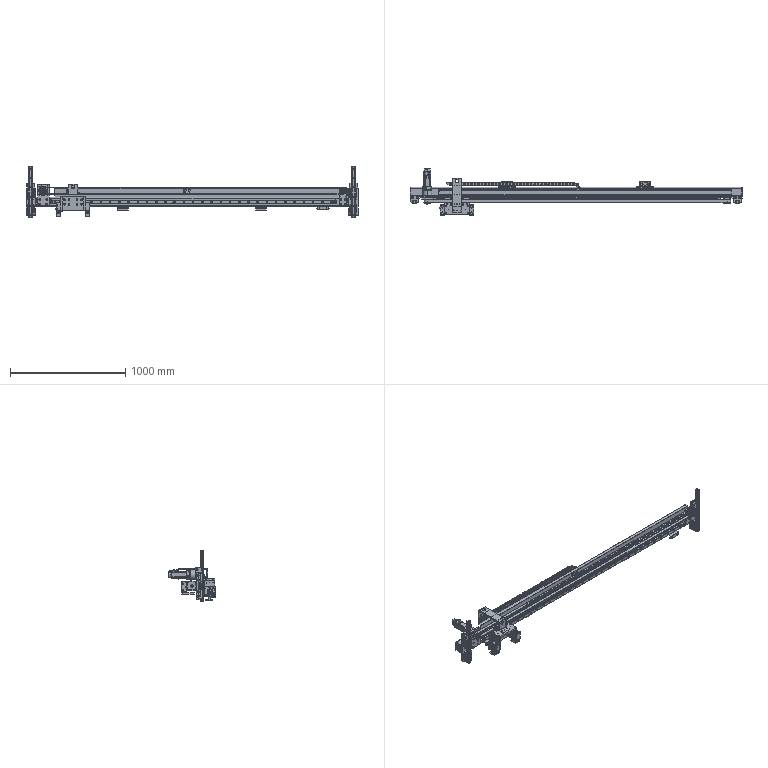Part | SolidWorks | 145 solids | 9464 faces | volume 16521485 mm3 | plane 4399 | cylinder 4181 | cone 721 | torus 116 | spline 38 | sphere 9 | commonest cylinder face diameters 1 x519 6 x444 6.8 x172 5.9 x168 1.1 x156 9 x154